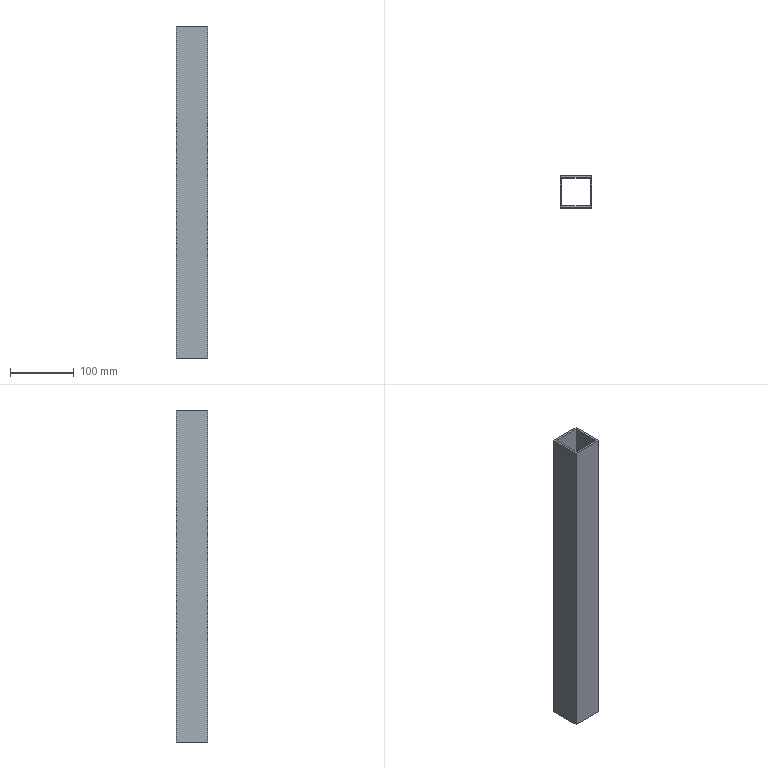Part | SolidWorks | features Extrusion 1 | 1 solid | 10 faces | box 50 x 50 x 520 mm | volume 293280 mm3 | plane 10
STEP:
#1=CARTESIAN_POINT('',(0.,0.,520.));
#2=VERTEX_POINT('',#1);
#3=CARTESIAN_POINT('',(50.,0.,520.));
#4=VERTEX_POINT('',#3);
#5=CARTESIAN_POINT('',(50.,0.,520.));
#6=DIRECTION('',(1.,0.,0.));
#7=VECTOR('',#6,1000.);
#8=LINE('',#5,#7);
#9=EDGE_CURVE('',#2,#4,#8,.T.);
#10=ORIENTED_EDGE('',*,*,#9,.T.);
#11=CARTESIAN_POINT('',(50.,50.,520.));
#12=VERTEX_POINT('',#11);
#13=CARTESIAN_POINT('',(50.,50.,520.));
#14=DIRECTION('',(0.,1.,0.));
#15=VECTOR('',#14,1000.);
#16=LINE('',#13,#15);
#17=EDGE_CURVE('',#4,#12,#16,.T.);
#18=ORIENTED_EDGE('',*,*,#17,.T.);
#19=CARTESIAN_POINT('',(0.,50.,520.));
#20=VERTEX_POINT('',#19);
#21=CARTESIAN_POINT('',(0.,50.,520.));
#22=DIRECTION('',(-1.,0.,0.));
#23=VECTOR('',#22,1000.);
#24=LINE('',#21,#23);
#25=EDGE_CURVE('',#12,#20,#24,.T.);
#26=ORIENTED_EDGE('',*,*,#25,.T.);
#27=CARTESIAN_POINT('',(0.,0.,520.));
#28=DIRECTION('',(0.,-1.,0.));
#29=VECTOR('',#28,1000.);
#30=LINE('',#27,#29);
#31=EDGE_CURVE('',#20,#2,#30,.T.);
#32=ORIENTED_EDGE('',*,*,#31,.T.);
#33=EDGE_LOOP('',(#10,#18,#26,#32));
#34=FACE_OUTER_BOUND('',#33,.T.);
#35=CARTESIAN_POINT('',(3.,3.,520.));
#36=VERTEX_POINT('',#35);
#37=CARTESIAN_POINT('',(47.,3.,520.));
#38=VERTEX_POINT('',#37);
#39=CARTESIAN_POINT('',(47.,3.,520.));
#40=DIRECTION('',(1.,0.,0.));
#41=VECTOR('',#40,1000.);
#42=LINE('',#39,#41);
#43=EDGE_CURVE('',#36,#38,#42,.T.);
#44=ORIENTED_EDGE('',*,*,#43,.F.);
#45=CARTESIAN_POINT('',(3.,47.,520.));
#46=VERTEX_POINT('',#45);
#47=CARTESIAN_POINT('',(3.,3.,520.));
#48=DIRECTION('',(0.,-1.,0.));
#49=VECTOR('',#48,1000.);
#50=LINE('',#47,#49);
#51=EDGE_CURVE('',#46,#36,#50,.T.);
#52=ORIENTED_EDGE('',*,*,#51,.F.);
#53=CARTESIAN_POINT('',(47.,47.,520.));
#54=VERTEX_POINT('',#53);
#55=CARTESIAN_POINT('',(3.,47.,520.));
#56=DIRECTION('',(-1.,0.,0.));
#57=VECTOR('',#56,1000.);
#58=LINE('',#55,#57);
#59=EDGE_CURVE('',#54,#46,#58,.T.);
#60=ORIENTED_EDGE('',*,*,#59,.F.);
#61=CARTESIAN_POINT('',(47.,47.,520.));
#62=DIRECTION('',(0.,1.,0.));
#63=VECTOR('',#62,1000.);
#64=LINE('',#61,#63);
#65=EDGE_CURVE('',#38,#54,#64,.T.);
#66=ORIENTED_EDGE('',*,*,#65,.F.);
#67=EDGE_LOOP('',(#44,#52,#60,#66));
#68=FACE_BOUND('',#67,.T.);
#69=CARTESIAN_POINT('',(0.,0.,520.));
#70=DIRECTION('',(0.,0.,-1.));
#71=DIRECTION('',(-1.,0.,0.));
#72=AXIS2_PLACEMENT_3D('',#69,#70,#71);
#73=PLANE('',#72);
#74=ADVANCED_FACE('',(#34,#68),#73,.F.);
#75=CARTESIAN_POINT('',(0.,0.,0.));
#76=VERTEX_POINT('',#75);
#77=CARTESIAN_POINT('',(50.,0.,0.));
#78=VERTEX_POINT('',#77);
#79=CARTESIAN_POINT('',(50.,0.,0.));
#80=DIRECTION('',(1.,0.,0.));
#81=VECTOR('',#80,1000.);
#82=LINE('',#79,#81);
#83=EDGE_CURVE('',#76,#78,#82,.T.);
#84=ORIENTED_EDGE('',*,*,#83,.F.);
#85=CARTESIAN_POINT('',(0.,50.,0.));
#86=VERTEX_POINT('',#85);
#87=CARTESIAN_POINT('',(0.,0.,0.));
#88=DIRECTION('',(0.,-1.,0.));
#89=VECTOR('',#88,1000.);
#90=LINE('',#87,#89);
#91=EDGE_CURVE('',#86,#76,#90,.T.);
#92=ORIENTED_EDGE('',*,*,#91,.F.);
#93=CARTESIAN_POINT('',(50.,50.,0.));
#94=VERTEX_POINT('',#93);
#95=CARTESIAN_POINT('',(0.,50.,0.));
#96=DIRECTION('',(-1.,0.,0.));
#97=VECTOR('',#96,1000.);
#98=LINE('',#95,#97);
#99=EDGE_CURVE('',#94,#86,#98,.T.);
#100=ORIENTED_EDGE('',*,*,#99,.F.);
#101=CARTESIAN_POINT('',(50.,50.,0.));
#102=DIRECTION('',(0.,1.,0.));
#103=VECTOR('',#102,1000.);
#104=LINE('',#101,#103);
#105=EDGE_CURVE('',#78,#94,#104,.T.);
#106=ORIENTED_EDGE('',*,*,#105,.F.);
#107=EDGE_LOOP('',(#84,#92,#100,#106));
#108=FACE_OUTER_BOUND('',#107,.T.);
#109=CARTESIAN_POINT('',(3.,47.,0.));
#110=VERTEX_POINT('',#109);
#111=CARTESIAN_POINT('',(3.,3.,0.));
#112=VERTEX_POINT('',#111);
#113=CARTESIAN_POINT('',(3.,3.,0.));
#114=DIRECTION('',(0.,-1.,0.));
#115=VECTOR('',#114,1000.);
#116=LINE('',#113,#115);
#117=EDGE_CURVE('',#110,#112,#116,.T.);
#118=ORIENTED_EDGE('',*,*,#117,.T.);
#119=CARTESIAN_POINT('',(47.,3.,0.));
#120=VERTEX_POINT('',#119);
#121=CARTESIAN_POINT('',(47.,3.,0.));
#122=DIRECTION('',(1.,0.,0.));
#123=VECTOR('',#122,1000.);
#124=LINE('',#121,#123);
#125=EDGE_CURVE('',#112,#120,#124,.T.);
#126=ORIENTED_EDGE('',*,*,#125,.T.);
#127=CARTESIAN_POINT('',(47.,47.,0.));
#128=VERTEX_POINT('',#127);
#129=CARTESIAN_POINT('',(47.,47.,0.));
#130=DIRECTION('',(0.,1.,0.));
#131=VECTOR('',#130,1000.);
#132=LINE('',#129,#131);
#133=EDGE_CURVE('',#120,#128,#132,.T.);
#134=ORIENTED_EDGE('',*,*,#133,.T.);
#135=CARTESIAN_POINT('',(3.,47.,0.));
#136=DIRECTION('',(-1.,0.,0.));
#137=VECTOR('',#136,1000.);
#138=LINE('',#135,#137);
#139=EDGE_CURVE('',#128,#110,#138,.T.);
#140=ORIENTED_EDGE('',*,*,#139,.T.);
#141=EDGE_LOOP('',(#118,#126,#134,#140));
#142=FACE_BOUND('',#141,.T.);
#143=CARTESIAN_POINT('',(0.,0.,0.));
#144=DIRECTION('',(0.,0.,-1.));
#145=DIRECTION('',(-1.,0.,0.));
#146=AXIS2_PLACEMENT_3D('',#143,#144,#145);
#147=PLANE('',#146);
#148=ADVANCED_FACE('',(#108,#142),#147,.T.);
#149=ORIENTED_EDGE('',*,*,#83,.T.);
#150=CARTESIAN_POINT('',(50.,0.,520.));
#151=DIRECTION('',(0.,0.,-1.));
#152=VECTOR('',#151,1000.);
#153=LINE('',#150,#152);
#154=EDGE_CURVE('',#4,#78,#153,.T.);
#155=ORIENTED_EDGE('',*,*,#154,.F.);
#156=ORIENTED_EDGE('',*,*,#9,.F.);
#157=CARTESIAN_POINT('',(0.,0.,520.));
#158=DIRECTION('',(0.,0.,-1.));
#159=VECTOR('',#158,1000.);
#160=LINE('',#157,#159);
#161=EDGE_CURVE('',#2,#76,#160,.T.);
#162=ORIENTED_EDGE('',*,*,#161,.T.);
#163=EDGE_LOOP('',(#149,#155,#156,#162));
#164=FACE_OUTER_BOUND('',#163,.T.);
#165=CARTESIAN_POINT('',(50.,0.,520.));
#166=DIRECTION('',(0.,1.,0.));
#167=DIRECTION('',(0.,0.,1.));
#168=AXIS2_PLACEMENT_3D('',#165,#166,#167);
#169=PLANE('',#168);
#170=ADVANCED_FACE('',(#164),#169,.F.);
#171=ORIENTED_EDGE('',*,*,#105,.T.);
#172=CARTESIAN_POINT('',(50.,50.,520.));
#173=DIRECTION('',(0.,0.,-1.));
#174=VECTOR('',#173,1000.);
#175=LINE('',#172,#174);
#176=EDGE_CURVE('',#12,#94,#175,.T.);
#177=ORIENTED_EDGE('',*,*,#176,.F.);
#178=ORIENTED_EDGE('',*,*,#17,.F.);
#179=ORIENTED_EDGE('',*,*,#154,.T.);
#180=EDGE_LOOP('',(#171,#177,#178,#179));
#181=FACE_OUTER_BOUND('',#180,.T.);
#182=CARTESIAN_POINT('',(50.,50.,520.));
#183=DIRECTION('',(-1.,0.,0.));
#184=DIRECTION('',(0.,0.,1.));
#185=AXIS2_PLACEMENT_3D('',#182,#183,#184);
#186=PLANE('',#185);
#187=ADVANCED_FACE('',(#181),#186,.F.);
#188=ORIENTED_EDGE('',*,*,#99,.T.);
#189=CARTESIAN_POINT('',(0.,50.,520.));
#190=DIRECTION('',(0.,0.,-1.));
#191=VECTOR('',#190,1000.);
#192=LINE('',#189,#191);
#193=EDGE_CURVE('',#20,#86,#192,.T.);
#194=ORIENTED_EDGE('',*,*,#193,.F.);
#195=ORIENTED_EDGE('',*,*,#25,.F.);
#196=ORIENTED_EDGE('',*,*,#176,.T.);
#197=EDGE_LOOP('',(#188,#194,#195,#196));
#198=FACE_OUTER_BOUND('',#197,.T.);
#199=CARTESIAN_POINT('',(0.,50.,520.));
#200=DIRECTION('',(0.,-1.,0.));
#201=DIRECTION('',(0.,0.,-1.));
#202=AXIS2_PLACEMENT_3D('',#199,#200,#201);
#203=PLANE('',#202);
#204=ADVANCED_FACE('',(#198),#203,.F.);
#205=ORIENTED_EDGE('',*,*,#91,.T.);
#206=ORIENTED_EDGE('',*,*,#161,.F.);
#207=ORIENTED_EDGE('',*,*,#31,.F.);
#208=ORIENTED_EDGE('',*,*,#193,.T.);
#209=EDGE_LOOP('',(#205,#206,#207,#208));
#210=FACE_OUTER_BOUND('',#209,.T.);
#211=CARTESIAN_POINT('',(0.,0.,520.));
#212=DIRECTION('',(1.,0.,0.));
#213=DIRECTION('',(0.,0.,-1.));
#214=AXIS2_PLACEMENT_3D('',#211,#212,#213);
#215=PLANE('',#214);
#216=ADVANCED_FACE('',(#210),#215,.F.);
#217=ORIENTED_EDGE('',*,*,#125,.F.);
#218=CARTESIAN_POINT('',(3.,3.,520.));
#219=DIRECTION('',(0.,0.,-1.));
#220=VECTOR('',#219,1000.);
#221=LINE('',#218,#220);
#222=EDGE_CURVE('',#36,#112,#221,.T.);
#223=ORIENTED_EDGE('',*,*,#222,.F.);
#224=ORIENTED_EDGE('',*,*,#43,.T.);
#225=CARTESIAN_POINT('',(47.,3.,520.));
#226=DIRECTION('',(0.,0.,-1.));
#227=VECTOR('',#226,1000.);
#228=LINE('',#225,#227);
#229=EDGE_CURVE('',#38,#120,#228,.T.);
#230=ORIENTED_EDGE('',*,*,#229,.T.);
#231=EDGE_LOOP('',(#217,#223,#224,#230));
#232=FACE_OUTER_BOUND('',#231,.T.);
#233=CARTESIAN_POINT('',(47.,3.,520.));
#234=DIRECTION('',(0.,1.,0.));
#235=DIRECTION('',(0.,0.,1.));
#236=AXIS2_PLACEMENT_3D('',#233,#234,#235);
#237=PLANE('',#236);
#238=ADVANCED_FACE('',(#232),#237,.T.);
#239=ORIENTED_EDGE('',*,*,#133,.F.);
#240=ORIENTED_EDGE('',*,*,#229,.F.);
#241=ORIENTED_EDGE('',*,*,#65,.T.);
#242=CARTESIAN_POINT('',(47.,47.,520.));
#243=DIRECTION('',(0.,0.,-1.));
#244=VECTOR('',#243,1000.);
#245=LINE('',#242,#244);
#246=EDGE_CURVE('',#54,#128,#245,.T.);
#247=ORIENTED_EDGE('',*,*,#246,.T.);
#248=EDGE_LOOP('',(#239,#240,#241,#247));
#249=FACE_OUTER_BOUND('',#248,.T.);
#250=CARTESIAN_POINT('',(47.,47.,520.));
#251=DIRECTION('',(-1.,0.,0.));
#252=DIRECTION('',(0.,0.,1.));
#253=AXIS2_PLACEMENT_3D('',#250,#251,#252);
#254=PLANE('',#253);
#255=ADVANCED_FACE('',(#249),#254,.T.);
#256=ORIENTED_EDGE('',*,*,#139,.F.);
#257=ORIENTED_EDGE('',*,*,#246,.F.);
#258=ORIENTED_EDGE('',*,*,#59,.T.);
#259=CARTESIAN_POINT('',(3.,47.,520.));
#260=DIRECTION('',(0.,0.,-1.));
#261=VECTOR('',#260,1000.);
#262=LINE('',#259,#261);
#263=EDGE_CURVE('',#46,#110,#262,.T.);
#264=ORIENTED_EDGE('',*,*,#263,.T.);
#265=EDGE_LOOP('',(#256,#257,#258,#264));
#266=FACE_OUTER_BOUND('',#265,.T.);
#267=CARTESIAN_POINT('',(3.,47.,520.));
#268=DIRECTION('',(0.,-1.,0.));
#269=DIRECTION('',(0.,0.,-1.));
#270=AXIS2_PLACEMENT_3D('',#267,#268,#269);
#271=PLANE('',#270);
#272=ADVANCED_FACE('',(#266),#271,.T.);
#273=ORIENTED_EDGE('',*,*,#117,.F.);
#274=ORIENTED_EDGE('',*,*,#263,.F.);
#275=ORIENTED_EDGE('',*,*,#51,.T.);
#276=ORIENTED_EDGE('',*,*,#222,.T.);
#277=EDGE_LOOP('',(#273,#274,#275,#276));
#278=FACE_OUTER_BOUND('',#277,.T.);
#279=CARTESIAN_POINT('',(3.,3.,520.));
#280=DIRECTION('',(1.,0.,0.));
#281=DIRECTION('',(0.,0.,-1.));
#282=AXIS2_PLACEMENT_3D('',#279,#280,#281);
#283=PLANE('',#282);
#284=ADVANCED_FACE('',(#278),#283,.T.);
#285=CLOSED_SHELL('',(#74,#148,#170,#187,#204,#216,#238,#255,#272,#284));
#286=MANIFOLD_SOLID_BREP('',#285);
#287=CARTESIAN_POINT('',(0.,0.,0.));
#288=DIRECTION('',(0.,0.,1.));
#289=DIRECTION('',(1.,0.,0.));
#290=AXIS2_PLACEMENT_3D('',#287,#288,#289);
#291=(LENGTH_UNIT()NAMED_UNIT(*)SI_UNIT(.MILLI.,.METRE.));
#292=UNCERTAINTY_MEASURE_WITH_UNIT(LENGTH_MEASURE(0.00001),#291,'','');
#293=(NAMED_UNIT(*)PLANE_ANGLE_UNIT()SI_UNIT($,.RADIAN.));
#294=(NAMED_UNIT(*)SI_UNIT($,.STERADIAN.)SOLID_ANGLE_UNIT());
#295=(GEOMETRIC_REPRESENTATION_CONTEXT(3)GLOBAL_UNCERTAINTY_ASSIGNED_CONTEXT((#292))GLOBAL_UNIT_ASSIGNED_CONTEXT((#291,#293,#294))REPRESENTATION_CONTEXT('',''));
#296=ADVANCED_BREP_SHAPE_REPRESENTATION('',(#286,#290),#295);